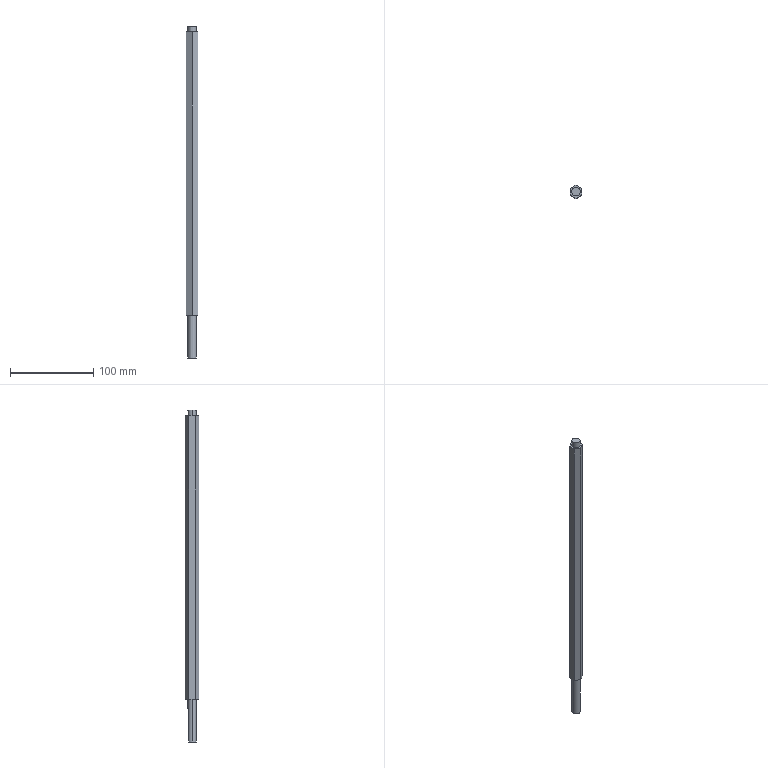Part | STEP file | 602-12-0050 | 1 solid | 16 faces | box 14 x 16.166 x 398 mm | volume 62104 mm3 | plane 12 | cylinder 4 | commonest cylinder face diameters 10 x4
STEP:
#1=CARTESIAN_POINT('',(0.,0.,0.));
#2=DIRECTION('',(0.,0.,1.));
#3=DIRECTION('',(1.,0.,0.));
#4=AXIS2_PLACEMENT_3D('',#1,#2,#3);
#5=CARTESIAN_POINT('',(-5.,0.,-51.));
#6=VERTEX_POINT('',#5);
#7=CARTESIAN_POINT('',(-3.,4.,-51.));
#8=VERTEX_POINT('',#7);
#9=CARTESIAN_POINT('',(0.,0.,-51.));
#10=DIRECTION('',(0.,0.,-1.));
#11=DIRECTION('',(-1.,0.,0.));
#12=AXIS2_PLACEMENT_3D('',#9,#10,#11);
#13=CIRCLE('',#12,5.);
#14=CARTESIAN_POINT('',(0.,0.,-51.));
#15=DIRECTION('',(0.,0.,1.));
#16=DIRECTION('',(1.,0.,0.));
#17=AXIS2_PLACEMENT_3D('',#14,#15,#16);
#18=CYLINDRICAL_SURFACE('',#17,5.);
#19=CARTESIAN_POINT('',(3.142,0.));
#20=DIRECTION('',(-1.,0.));
#21=VECTOR('',#20,1.);
#22=LINE('',#19,#21);
#23=(GEOMETRIC_REPRESENTATION_CONTEXT(2)PARAMETRIC_REPRESENTATION_CONTEXT()REPRESENTATION_CONTEXT('',''));
#24=DEFINITIONAL_REPRESENTATION('',(#22),#23);
#25=PCURVE('',#18,#24);
#26=CARTESIAN_POINT('',(0.,0.,-51.));
#27=DIRECTION('',(0.,0.,-1.));
#28=DIRECTION('',(-1.,0.,0.));
#29=AXIS2_PLACEMENT_3D('',#26,#27,#28);
#30=PLANE('',#29);
#31=CARTESIAN_POINT('',(0.,0.));
#32=DIRECTION('',(1.,0.));
#33=AXIS2_PLACEMENT_2D('',#31,#32);
#34=CIRCLE('',#33,5.);
#35=(GEOMETRIC_REPRESENTATION_CONTEXT(2)PARAMETRIC_REPRESENTATION_CONTEXT()REPRESENTATION_CONTEXT('',''));
#36=DEFINITIONAL_REPRESENTATION('',(#34),#35);
#37=PCURVE('',#30,#36);
#38=SURFACE_CURVE('',#13,(#25,#37),.PCURVE_S1.);
#39=EDGE_CURVE('',#6,#8,#38,.T.);
#40=ORIENTED_EDGE('',*,*,#39,.F.);
#41=CARTESIAN_POINT('',(-5.,0.,0.));
#42=VERTEX_POINT('',#41);
#43=CARTESIAN_POINT('',(-5.,0.,-51.));
#44=DIRECTION('',(0.,0.,1.));
#45=VECTOR('',#44,1.);
#46=LINE('',#43,#45);
#47=CARTESIAN_POINT('',(3.142,0.));
#48=DIRECTION('',(0.,1.));
#49=VECTOR('',#48,1.);
#50=LINE('',#47,#49);
#51=(GEOMETRIC_REPRESENTATION_CONTEXT(2)PARAMETRIC_REPRESENTATION_CONTEXT()REPRESENTATION_CONTEXT('',''));
#52=DEFINITIONAL_REPRESENTATION('',(#50),#51);
#53=PCURVE('',#18,#52);
#54=CARTESIAN_POINT('',(0.,0.,-51.));
#55=DIRECTION('',(0.,0.,1.));
#56=DIRECTION('',(1.,0.,0.));
#57=AXIS2_PLACEMENT_3D('',#54,#55,#56);
#58=CYLINDRICAL_SURFACE('',#57,5.);
#59=CARTESIAN_POINT('',(3.142,0.));
#60=DIRECTION('',(0.,1.));
#61=VECTOR('',#60,1.);
#62=LINE('',#59,#61);
#63=(GEOMETRIC_REPRESENTATION_CONTEXT(2)PARAMETRIC_REPRESENTATION_CONTEXT()REPRESENTATION_CONTEXT('',''));
#64=DEFINITIONAL_REPRESENTATION('',(#62),#63);
#65=PCURVE('',#58,#64);
#66=SURFACE_CURVE('',#46,(#53,#65),.PCURVE_S1.);
#67=EDGE_CURVE('',#6,#42,#66,.T.);
#68=ORIENTED_EDGE('',*,*,#67,.T.);
#69=CARTESIAN_POINT('',(5.,0.,0.));
#70=VERTEX_POINT('',#69);
#71=CARTESIAN_POINT('',(0.,0.,0.));
#72=DIRECTION('',(0.,0.,-1.));
#73=DIRECTION('',(1.,0.,0.));
#74=AXIS2_PLACEMENT_3D('',#71,#72,#73);
#75=CIRCLE('',#74,5.);
#76=CARTESIAN_POINT('',(6.283,51.));
#77=DIRECTION('',(-1.,0.));
#78=VECTOR('',#77,1.);
#79=LINE('',#76,#78);
#80=(GEOMETRIC_REPRESENTATION_CONTEXT(2)PARAMETRIC_REPRESENTATION_CONTEXT()REPRESENTATION_CONTEXT('',''));
#81=DEFINITIONAL_REPRESENTATION('',(#79),#80);
#82=PCURVE('',#18,#81);
#83=CARTESIAN_POINT('',(0.,0.,0.));
#84=DIRECTION('',(0.,0.,1.));
#85=DIRECTION('',(1.,0.,0.));
#86=AXIS2_PLACEMENT_3D('',#83,#84,#85);
#87=PLANE('',#86);
#88=CARTESIAN_POINT('',(5.,0.));
#89=CARTESIAN_POINT('',(5.,-8.66));
#90=CARTESIAN_POINT('',(-2.5,-4.33));
#91=CARTESIAN_POINT('',(-10.,0.));
#92=CARTESIAN_POINT('',(-2.5,4.33));
#93=CARTESIAN_POINT('',(5.,8.66));
#94=CARTESIAN_POINT('',(5.,0.));
#95=(BOUNDED_CURVE()B_SPLINE_CURVE(2,(#88,#89,#90,#91,#92,#93,#94),.UNSPECIFIED.,.T.,.F.)B_SPLINE_CURVE_WITH_KNOTS((1,2,2,2,2,1),(-2.094,0.,2.094,4.189,6.283,8.378),.UNSPECIFIED.)CURVE()GEOMETRIC_REPRESENTATION_ITEM()RATIONAL_B_SPLINE_CURVE((1.,0.5,1.,0.5,1.,0.5,1.))REPRESENTATION_ITEM(''));
#96=(GEOMETRIC_REPRESENTATION_CONTEXT(2)PARAMETRIC_REPRESENTATION_CONTEXT()REPRESENTATION_CONTEXT('',''));
#97=DEFINITIONAL_REPRESENTATION('',(#95),#96);
#98=PCURVE('',#87,#97);
#99=SURFACE_CURVE('',#75,(#82,#98),.PCURVE_S1.);
#100=EDGE_CURVE('',#42,#70,#99,.T.);
#101=ORIENTED_EDGE('',*,*,#100,.T.);
#102=CARTESIAN_POINT('',(5.,0.,-51.));
#103=VERTEX_POINT('',#102);
#104=CARTESIAN_POINT('',(5.,0.,-51.));
#105=DIRECTION('',(0.,0.,1.));
#106=VECTOR('',#105,1.);
#107=LINE('',#104,#106);
#108=CARTESIAN_POINT('',(0.,0.));
#109=DIRECTION('',(0.,1.));
#110=VECTOR('',#109,1.);
#111=LINE('',#108,#110);
#112=(GEOMETRIC_REPRESENTATION_CONTEXT(2)PARAMETRIC_REPRESENTATION_CONTEXT()REPRESENTATION_CONTEXT('',''));
#113=DEFINITIONAL_REPRESENTATION('',(#111),#112);
#114=PCURVE('',#18,#113);
#115=CARTESIAN_POINT('',(6.283,0.));
#116=DIRECTION('',(0.,1.));
#117=VECTOR('',#116,1.);
#118=LINE('',#115,#117);
#119=(GEOMETRIC_REPRESENTATION_CONTEXT(2)PARAMETRIC_REPRESENTATION_CONTEXT()REPRESENTATION_CONTEXT('',''));
#120=DEFINITIONAL_REPRESENTATION('',(#118),#119);
#121=PCURVE('',#58,#120);
#122=SURFACE_CURVE('',#107,(#114,#121),.PCURVE_S1.);
#123=EDGE_CURVE('',#103,#70,#122,.T.);
#124=ORIENTED_EDGE('',*,*,#123,.F.);
#125=CARTESIAN_POINT('',(3.,4.,-51.));
#126=VERTEX_POINT('',#125);
#127=CARTESIAN_POINT('',(0.,0.,-51.));
#128=DIRECTION('',(0.,0.,-1.));
#129=DIRECTION('',(-1.,0.,0.));
#130=AXIS2_PLACEMENT_3D('',#127,#128,#129);
#131=CIRCLE('',#130,5.);
#132=CARTESIAN_POINT('',(3.142,0.));
#133=DIRECTION('',(-1.,0.));
#134=VECTOR('',#133,1.);
#135=LINE('',#132,#134);
#136=(GEOMETRIC_REPRESENTATION_CONTEXT(2)PARAMETRIC_REPRESENTATION_CONTEXT()REPRESENTATION_CONTEXT('',''));
#137=DEFINITIONAL_REPRESENTATION('',(#135),#136);
#138=PCURVE('',#18,#137);
#139=CARTESIAN_POINT('',(0.,0.));
#140=DIRECTION('',(1.,0.));
#141=AXIS2_PLACEMENT_2D('',#139,#140);
#142=CIRCLE('',#141,5.);
#143=(GEOMETRIC_REPRESENTATION_CONTEXT(2)PARAMETRIC_REPRESENTATION_CONTEXT()REPRESENTATION_CONTEXT('',''));
#144=DEFINITIONAL_REPRESENTATION('',(#142),#143);
#145=PCURVE('',#30,#144);
#146=SURFACE_CURVE('',#131,(#138,#145),.PCURVE_S1.);
#147=EDGE_CURVE('',#126,#103,#146,.T.);
#148=ORIENTED_EDGE('',*,*,#147,.F.);
#149=CARTESIAN_POINT('',(3.,4.,-11.));
#150=VERTEX_POINT('',#149);
#151=CARTESIAN_POINT('',(3.,4.,-11.));
#152=DIRECTION('',(0.,0.,-1.));
#153=VECTOR('',#152,1.);
#154=LINE('',#151,#153);
#155=CARTESIAN_POINT('',(0.9273,40.));
#156=DIRECTION('',(0.,-1.));
#157=VECTOR('',#156,1.);
#158=LINE('',#155,#157);
#159=(GEOMETRIC_REPRESENTATION_CONTEXT(2)PARAMETRIC_REPRESENTATION_CONTEXT()REPRESENTATION_CONTEXT('',''));
#160=DEFINITIONAL_REPRESENTATION('',(#158),#159);
#161=PCURVE('',#18,#160);
#162=CARTESIAN_POINT('',(3.,4.,-11.));
#163=DIRECTION('',(0.,-1.,0.));
#164=DIRECTION('',(0.,0.,-1.));
#165=AXIS2_PLACEMENT_3D('',#162,#163,#164);
#166=PLANE('',#165);
#167=CARTESIAN_POINT('',(0.,0.));
#168=DIRECTION('',(1.,0.));
#169=VECTOR('',#168,1.);
#170=LINE('',#167,#169);
#171=(GEOMETRIC_REPRESENTATION_CONTEXT(2)PARAMETRIC_REPRESENTATION_CONTEXT()REPRESENTATION_CONTEXT('',''));
#172=DEFINITIONAL_REPRESENTATION('',(#170),#171);
#173=PCURVE('',#166,#172);
#174=SURFACE_CURVE('',#154,(#161,#173),.PCURVE_S1.);
#175=EDGE_CURVE('',#150,#126,#174,.T.);
#176=ORIENTED_EDGE('',*,*,#175,.F.);
#177=CARTESIAN_POINT('',(-3.,4.,-11.));
#178=VERTEX_POINT('',#177);
#179=CARTESIAN_POINT('',(0.,0.,-11.));
#180=DIRECTION('',(0.,0.,-1.));
#181=DIRECTION('',(-1.,0.,0.));
#182=AXIS2_PLACEMENT_3D('',#179,#180,#181);
#183=CIRCLE('',#182,5.);
#184=CARTESIAN_POINT('',(3.142,40.));
#185=DIRECTION('',(-1.,0.));
#186=VECTOR('',#185,1.);
#187=LINE('',#184,#186);
#188=(GEOMETRIC_REPRESENTATION_CONTEXT(2)PARAMETRIC_REPRESENTATION_CONTEXT()REPRESENTATION_CONTEXT('',''));
#189=DEFINITIONAL_REPRESENTATION('',(#187),#188);
#190=PCURVE('',#18,#189);
#191=CARTESIAN_POINT('',(0.,0.,-11.));
#192=DIRECTION('',(0.,0.,-1.));
#193=DIRECTION('',(-1.,0.,0.));
#194=AXIS2_PLACEMENT_3D('',#191,#192,#193);
#195=PLANE('',#194);
#196=CARTESIAN_POINT('',(0.,0.));
#197=DIRECTION('',(1.,0.));
#198=AXIS2_PLACEMENT_2D('',#196,#197);
#199=CIRCLE('',#198,5.);
#200=(GEOMETRIC_REPRESENTATION_CONTEXT(2)PARAMETRIC_REPRESENTATION_CONTEXT()REPRESENTATION_CONTEXT('',''));
#201=DEFINITIONAL_REPRESENTATION('',(#199),#200);
#202=PCURVE('',#195,#201);
#203=SURFACE_CURVE('',#183,(#190,#202),.PCURVE_S1.);
#204=EDGE_CURVE('',#178,#150,#203,.T.);
#205=ORIENTED_EDGE('',*,*,#204,.F.);
#206=CARTESIAN_POINT('',(-3.,4.,-11.));
#207=DIRECTION('',(0.,0.,-1.));
#208=VECTOR('',#207,1.);
#209=LINE('',#206,#208);
#210=CARTESIAN_POINT('',(2.214,40.));
#211=DIRECTION('',(0.,-1.));
#212=VECTOR('',#211,1.);
#213=LINE('',#210,#212);
#214=(GEOMETRIC_REPRESENTATION_CONTEXT(2)PARAMETRIC_REPRESENTATION_CONTEXT()REPRESENTATION_CONTEXT('',''));
#215=DEFINITIONAL_REPRESENTATION('',(#213),#214);
#216=PCURVE('',#18,#215);
#217=CARTESIAN_POINT('',(0.,-6.));
#218=DIRECTION('',(1.,0.));
#219=VECTOR('',#218,1.);
#220=LINE('',#217,#219);
#221=(GEOMETRIC_REPRESENTATION_CONTEXT(2)PARAMETRIC_REPRESENTATION_CONTEXT()REPRESENTATION_CONTEXT('',''));
#222=DEFINITIONAL_REPRESENTATION('',(#220),#221);
#223=PCURVE('',#166,#222);
#224=SURFACE_CURVE('',#209,(#216,#223),.PCURVE_S1.);
#225=EDGE_CURVE('',#178,#8,#224,.T.);
#226=ORIENTED_EDGE('',*,*,#225,.T.);
#227=EDGE_LOOP('',(#40,#68,#101,#124,#148,#176,#205,#226));
#228=FACE_BOUND('',#227,.T.);
#229=ADVANCED_FACE('',(#228),#18,.T.);
#230=CARTESIAN_POINT('',(5.,0.,347.));
#231=VERTEX_POINT('',#230);
#232=CARTESIAN_POINT('',(-5.,0.,347.));
#233=VERTEX_POINT('',#232);
#234=CARTESIAN_POINT('',(0.,0.,347.));
#235=DIRECTION('',(0.,0.,1.));
#236=DIRECTION('',(1.,0.,0.));
#237=AXIS2_PLACEMENT_3D('',#234,#235,#236);
#238=CIRCLE('',#237,5.);
#239=CARTESIAN_POINT('',(0.,0.,347.));
#240=DIRECTION('',(0.,0.,-1.));
#241=DIRECTION('',(-1.,0.,0.));
#242=AXIS2_PLACEMENT_3D('',#239,#240,#241);
#243=CYLINDRICAL_SURFACE('',#242,5.);
#244=CARTESIAN_POINT('',(3.142,0.));
#245=DIRECTION('',(-1.,0.));
#246=VECTOR('',#245,1.);
#247=LINE('',#244,#246);
#248=(GEOMETRIC_REPRESENTATION_CONTEXT(2)PARAMETRIC_REPRESENTATION_CONTEXT()REPRESENTATION_CONTEXT('',''));
#249=DEFINITIONAL_REPRESENTATION('',(#247),#248);
#250=PCURVE('',#243,#249);
#251=CARTESIAN_POINT('',(0.,0.,347.));
#252=DIRECTION('',(0.,0.,1.));
#253=DIRECTION('',(1.,0.,0.));
#254=AXIS2_PLACEMENT_3D('',#251,#252,#253);
#255=PLANE('',#254);
#256=CARTESIAN_POINT('',(0.,0.));
#257=DIRECTION('',(1.,0.));
#258=AXIS2_PLACEMENT_2D('',#256,#257);
#259=CIRCLE('',#258,5.);
#260=(GEOMETRIC_REPRESENTATION_CONTEXT(2)PARAMETRIC_REPRESENTATION_CONTEXT()REPRESENTATION_CONTEXT('',''));
#261=DEFINITIONAL_REPRESENTATION('',(#259),#260);
#262=PCURVE('',#255,#261);
#263=SURFACE_CURVE('',#238,(#250,#262),.PCURVE_S1.);
#264=EDGE_CURVE('',#231,#233,#263,.T.);
#265=ORIENTED_EDGE('',*,*,#264,.F.);
#266=CARTESIAN_POINT('',(5.,0.,340.));
#267=VERTEX_POINT('',#266);
#268=CARTESIAN_POINT('',(5.,0.,347.));
#269=DIRECTION('',(0.,0.,-1.));
#270=VECTOR('',#269,1.);
#271=LINE('',#268,#270);
#272=CARTESIAN_POINT('',(3.142,0.));
#273=DIRECTION('',(0.,1.));
#274=VECTOR('',#273,1.);
#275=LINE('',#272,#274);
#276=(GEOMETRIC_REPRESENTATION_CONTEXT(2)PARAMETRIC_REPRESENTATION_CONTEXT()REPRESENTATION_CONTEXT('',''));
#277=DEFINITIONAL_REPRESENTATION('',(#275),#276);
#278=PCURVE('',#243,#277);
#279=CARTESIAN_POINT('',(0.,0.,347.));
#280=DIRECTION('',(0.,0.,-1.));
#281=DIRECTION('',(-1.,0.,0.));
#282=AXIS2_PLACEMENT_3D('',#279,#280,#281);
#283=CYLINDRICAL_SURFACE('',#282,5.);
#284=CARTESIAN_POINT('',(3.142,0.));
#285=DIRECTION('',(0.,1.));
#286=VECTOR('',#285,1.);
#287=LINE('',#284,#286);
#288=(GEOMETRIC_REPRESENTATION_CONTEXT(2)PARAMETRIC_REPRESENTATION_CONTEXT()REPRESENTATION_CONTEXT('',''));
#289=DEFINITIONAL_REPRESENTATION('',(#287),#288);
#290=PCURVE('',#283,#289);
#291=SURFACE_CURVE('',#271,(#278,#290),.PCURVE_S1.);
#292=EDGE_CURVE('',#231,#267,#291,.T.);
#293=ORIENTED_EDGE('',*,*,#292,.T.);
#294=CARTESIAN_POINT('',(-5.,0.,340.));
#295=VERTEX_POINT('',#294);
#296=CARTESIAN_POINT('',(0.,0.,340.));
#297=DIRECTION('',(0.,0.,1.));
#298=DIRECTION('',(1.,0.,0.));
#299=AXIS2_PLACEMENT_3D('',#296,#297,#298);
#300=CIRCLE('',#299,5.);
#301=CARTESIAN_POINT('',(3.142,7.));
#302=DIRECTION('',(-1.,0.));
#303=VECTOR('',#302,1.);
#304=LINE('',#301,#303);
#305=(GEOMETRIC_REPRESENTATION_CONTEXT(2)PARAMETRIC_REPRESENTATION_CONTEXT()REPRESENTATION_CONTEXT('',''));
#306=DEFINITIONAL_REPRESENTATION('',(#304),#305);
#307=PCURVE('',#243,#306);
#308=CARTESIAN_POINT('',(0.,0.,340.));
#309=DIRECTION('',(0.,0.,1.));
#310=DIRECTION('',(1.,0.,0.));
#311=AXIS2_PLACEMENT_3D('',#308,#309,#310);
#312=PLANE('',#311);
#313=CARTESIAN_POINT('',(0.,0.));
#314=DIRECTION('',(1.,0.));
#315=AXIS2_PLACEMENT_2D('',#313,#314);
#316=CIRCLE('',#315,5.);
#317=(GEOMETRIC_REPRESENTATION_CONTEXT(2)PARAMETRIC_REPRESENTATION_CONTEXT()REPRESENTATION_CONTEXT('',''));
#318=DEFINITIONAL_REPRESENTATION('',(#316),#317);
#319=PCURVE('',#312,#318);
#320=SURFACE_CURVE('',#300,(#307,#319),.PCURVE_S1.);
#321=EDGE_CURVE('',#267,#295,#320,.T.);
#322=ORIENTED_EDGE('',*,*,#321,.T.);
#323=CARTESIAN_POINT('',(-5.,0.,347.));
#324=DIRECTION('',(0.,0.,-1.));
#325=VECTOR('',#324,1.);
#326=LINE('',#323,#325);
#327=CARTESIAN_POINT('',(0.,0.));
#328=DIRECTION('',(0.,1.));
#329=VECTOR('',#328,1.);
#330=LINE('',#327,#329);
#331=(GEOMETRIC_REPRESENTATION_CONTEXT(2)PARAMETRIC_REPRESENTATION_CONTEXT()REPRESENTATION_CONTEXT('',''));
#332=DEFINITIONAL_REPRESENTATION('',(#330),#331);
#333=PCURVE('',#243,#332);
#334=CARTESIAN_POINT('',(6.283,0.));
#335=DIRECTION('',(0.,1.));
#336=VECTOR('',#335,1.);
#337=LINE('',#334,#336);
#338=(GEOMETRIC_REPRESENTATION_CONTEXT(2)PARAMETRIC_REPRESENTATION_CONTEXT()REPRESENTATION_CONTEXT('',''));
#339=DEFINITIONAL_REPRESENTATION('',(#337),#338);
#340=PCURVE('',#283,#339);
#341=SURFACE_CURVE('',#326,(#333,#340),.PCURVE_S1.);
#342=EDGE_CURVE('',#233,#295,#341,.T.);
#343=ORIENTED_EDGE('',*,*,#342,.F.);
#344=EDGE_LOOP('',(#265,#293,#322,#343));
#345=FACE_BOUND('',#344,.T.);
#346=ADVANCED_FACE('',(#345),#243,.T.);
#347=CARTESIAN_POINT('',(7.,4.041,0.));
#348=VERTEX_POINT('',#347);
#349=CARTESIAN_POINT('',(0.,8.083,0.));
#350=VERTEX_POINT('',#349);
#351=CARTESIAN_POINT('',(7.,4.041,0.));
#352=DIRECTION('',(-0.866,0.5,0.));
#353=VECTOR('',#352,1.);
#354=LINE('',#351,#353);
#355=CARTESIAN_POINT('',(7.,4.041));
#356=DIRECTION('',(-0.866,0.5));
#357=VECTOR('',#356,1.);
#358=LINE('',#355,#357);
#359=(GEOMETRIC_REPRESENTATION_CONTEXT(2)PARAMETRIC_REPRESENTATION_CONTEXT()REPRESENTATION_CONTEXT('',''));
#360=DEFINITIONAL_REPRESENTATION('',(#358),#359);
#361=PCURVE('',#87,#360);
#362=CARTESIAN_POINT('',(7.,4.041,340.));
#363=DIRECTION('',(-0.5,-0.866,0.));
#364=DIRECTION('',(0.866,-0.5,0.));
#365=AXIS2_PLACEMENT_3D('',#362,#363,#364);
#366=PLANE('',#365);
#367=CARTESIAN_POINT('',(0.,-340.));
#368=DIRECTION('',(-1.,0.));
#369=VECTOR('',#368,1.);
#370=LINE('',#367,#369);
#371=(GEOMETRIC_REPRESENTATION_CONTEXT(2)PARAMETRIC_REPRESENTATION_CONTEXT()REPRESENTATION_CONTEXT('',''));
#372=DEFINITIONAL_REPRESENTATION('',(#370),#371);
#373=PCURVE('',#366,#372);
#374=SURFACE_CURVE('',#354,(#361,#373),.PCURVE_S1.);
#375=EDGE_CURVE('',#348,#350,#374,.T.);
#376=ORIENTED_EDGE('',*,*,#375,.F.);
#377=CARTESIAN_POINT('',(7.,-4.041,0.));
#378=VERTEX_POINT('',#377);
#379=CARTESIAN_POINT('',(7.,-4.041,0.));
#380=DIRECTION('',(0.,1.,0.));
#381=VECTOR('',#380,1.);
#382=LINE('',#379,#381);
#383=CARTESIAN_POINT('',(7.,-4.041));
#384=DIRECTION('',(0.,1.));
#385=VECTOR('',#384,1.);
#386=LINE('',#383,#385);
#387=(GEOMETRIC_REPRESENTATION_CONTEXT(2)PARAMETRIC_REPRESENTATION_CONTEXT()REPRESENTATION_CONTEXT('',''));
#388=DEFINITIONAL_REPRESENTATION('',(#386),#387);
#389=PCURVE('',#87,#388);
#390=CARTESIAN_POINT('',(7.,-4.041,340.));
#391=DIRECTION('',(-1.,0.,0.));
#392=DIRECTION('',(0.,0.,1.));
#393=AXIS2_PLACEMENT_3D('',#390,#391,#392);
#394=PLANE('',#393);
#395=CARTESIAN_POINT('',(-340.,0.));
#396=DIRECTION('',(0.,1.));
#397=VECTOR('',#396,1.);
#398=LINE('',#395,#397);
#399=(GEOMETRIC_REPRESENTATION_CONTEXT(2)PARAMETRIC_REPRESENTATION_CONTEXT()REPRESENTATION_CONTEXT('',''));
#400=DEFINITIONAL_REPRESENTATION('',(#398),#399);
#401=PCURVE('',#394,#400);
#402=SURFACE_CURVE('',#382,(#389,#401),.PCURVE_S1.);
#403=EDGE_CURVE('',#378,#348,#402,.T.);
#404=ORIENTED_EDGE('',*,*,#403,.F.);
#405=CARTESIAN_POINT('',(0.,-8.083,0.));
#406=VERTEX_POINT('',#405);
#407=CARTESIAN_POINT('',(0.,-8.083,0.));
#408=DIRECTION('',(0.866,0.5,0.));
#409=VECTOR('',#408,1.);
#410=LINE('',#407,#409);
#411=CARTESIAN_POINT('',(0.,-8.083));
#412=DIRECTION('',(0.866,0.5));
#413=VECTOR('',#412,1.);
#414=LINE('',#411,#413);
#415=(GEOMETRIC_REPRESENTATION_CONTEXT(2)PARAMETRIC_REPRESENTATION_CONTEXT()REPRESENTATION_CONTEXT('',''));
#416=DEFINITIONAL_REPRESENTATION('',(#414),#415);
#417=PCURVE('',#87,#416);
#418=CARTESIAN_POINT('',(0.,-8.083,340.));
#419=DIRECTION('',(-0.5,0.866,0.));
#420=DIRECTION('',(-0.866,-0.5,0.));
#421=AXIS2_PLACEMENT_3D('',#418,#419,#420);
#422=PLANE('',#421);
#423=CARTESIAN_POINT('',(0.,-340.));
#424=DIRECTION('',(-1.,0.));
#425=VECTOR('',#424,1.);
#426=LINE('',#423,#425);
#427=(GEOMETRIC_REPRESENTATION_CONTEXT(2)PARAMETRIC_REPRESENTATION_CONTEXT()REPRESENTATION_CONTEXT('',''));
#428=DEFINITIONAL_REPRESENTATION('',(#426),#427);
#429=PCURVE('',#422,#428);
#430=SURFACE_CURVE('',#410,(#417,#429),.PCURVE_S1.);
#431=EDGE_CURVE('',#406,#378,#430,.T.);
#432=ORIENTED_EDGE('',*,*,#431,.F.);
#433=CARTESIAN_POINT('',(-7.,-4.041,0.));
#434=VERTEX_POINT('',#433);
#435=CARTESIAN_POINT('',(-7.,-4.041,0.));
#436=DIRECTION('',(0.866,-0.5,0.));
#437=VECTOR('',#436,1.);
#438=LINE('',#435,#437);
#439=CARTESIAN_POINT('',(-7.,-4.041));
#440=DIRECTION('',(0.866,-0.5));
#441=VECTOR('',#440,1.);
#442=LINE('',#439,#441);
#443=(GEOMETRIC_REPRESENTATION_CONTEXT(2)PARAMETRIC_REPRESENTATION_CONTEXT()REPRESENTATION_CONTEXT('',''));
#444=DEFINITIONAL_REPRESENTATION('',(#442),#443);
#445=PCURVE('',#87,#444);
#446=CARTESIAN_POINT('',(-7.,-4.041,340.));
#447=DIRECTION('',(0.5,0.866,0.));
#448=DIRECTION('',(-0.866,0.5,0.));
#449=AXIS2_PLACEMENT_3D('',#446,#447,#448);
#450=PLANE('',#449);
#451=CARTESIAN_POINT('',(0.,-340.));
#452=DIRECTION('',(-1.,0.));
#453=VECTOR('',#452,1.);
#454=LINE('',#451,#453);
#455=(GEOMETRIC_REPRESENTATION_CONTEXT(2)PARAMETRIC_REPRESENTATION_CONTEXT()REPRESENTATION_CONTEXT('',''));
#456=DEFINITIONAL_REPRESENTATION('',(#454),#455);
#457=PCURVE('',#450,#456);
#458=SURFACE_CURVE('',#438,(#445,#457),.PCURVE_S1.);
#459=EDGE_CURVE('',#434,#406,#458,.T.);
#460=ORIENTED_EDGE('',*,*,#459,.F.);
#461=CARTESIAN_POINT('',(-7.,4.041,0.));
#462=VERTEX_POINT('',#461);
#463=CARTESIAN_POINT('',(-7.,4.041,0.));
#464=DIRECTION('',(0.,-1.,0.));
#465=VECTOR('',#464,1.);
#466=LINE('',#463,#465);
#467=CARTESIAN_POINT('',(-7.,4.041));
#468=DIRECTION('',(0.,-1.));
#469=VECTOR('',#468,1.);
#470=LINE('',#467,#469);
#471=(GEOMETRIC_REPRESENTATION_CONTEXT(2)PARAMETRIC_REPRESENTATION_CONTEXT()REPRESENTATION_CONTEXT('',''));
#472=DEFINITIONAL_REPRESENTATION('',(#470),#471);
#473=PCURVE('',#87,#472);
#474=CARTESIAN_POINT('',(-7.,4.041,340.));
#475=DIRECTION('',(1.,0.,0.));
#476=DIRECTION('',(0.,0.,-1.));
#477=AXIS2_PLACEMENT_3D('',#474,#475,#476);
#478=PLANE('',#477);
#479=CARTESIAN_POINT('',(340.,0.));
#480=DIRECTION('',(0.,-1.));
#481=VECTOR('',#480,1.);
#482=LINE('',#479,#481);
#483=(GEOMETRIC_REPRESENTATION_CONTEXT(2)PARAMETRIC_REPRESENTATION_CONTEXT()REPRESENTATION_CONTEXT('',''));
#484=DEFINITIONAL_REPRESENTATION('',(#482),#483);
#485=PCURVE('',#478,#484);
#486=SURFACE_CURVE('',#466,(#473,#485),.PCURVE_S1.);
#487=EDGE_CURVE('',#462,#434,#486,.T.);
#488=ORIENTED_EDGE('',*,*,#487,.F.);
#489=CARTESIAN_POINT('',(0.,8.083,0.));
#490=DIRECTION('',(-0.866,-0.5,0.));
#491=VECTOR('',#490,1.);
#492=LINE('',#489,#491);
#493=CARTESIAN_POINT('',(0.,8.083));
#494=DIRECTION('',(-0.866,-0.5));
#495=VECTOR('',#494,1.);
#496=LINE('',#493,#495);
#497=(GEOMETRIC_REPRESENTATION_CONTEXT(2)PARAMETRIC_REPRESENTATION_CONTEXT()REPRESENTATION_CONTEXT('',''));
#498=DEFINITIONAL_REPRESENTATION('',(#496),#497);
#499=PCURVE('',#87,#498);
#500=CARTESIAN_POINT('',(0.,8.083,340.));
#501=DIRECTION('',(0.5,-0.866,0.));
#502=DIRECTION('',(0.866,0.5,0.));
#503=AXIS2_PLACEMENT_3D('',#500,#501,#502);
#504=PLANE('',#503);
#505=CARTESIAN_POINT('',(0.,-340.));
#506=DIRECTION('',(-1.,0.));
#507=VECTOR('',#506,1.);
#508=LINE('',#505,#507);
#509=(GEOMETRIC_REPRESENTATION_CONTEXT(2)PARAMETRIC_REPRESENTATION_CONTEXT()REPRESENTATION_CONTEXT('',''));
#510=DEFINITIONAL_REPRESENTATION('',(#508),#509);
#511=PCURVE('',#504,#510);
#512=SURFACE_CURVE('',#492,(#499,#511),.PCURVE_S1.);
#513=EDGE_CURVE('',#350,#462,#512,.T.);
#514=ORIENTED_EDGE('',*,*,#513,.F.);
#515=EDGE_LOOP('',(#376,#404,#432,#460,#488,#514));
#516=FACE_BOUND('',#515,.T.);
#517=CARTESIAN_POINT('',(0.,0.,0.));
#518=DIRECTION('',(0.,0.,-1.));
#519=DIRECTION('',(1.,0.,0.));
#520=AXIS2_PLACEMENT_3D('',#517,#518,#519);
#521=CIRCLE('',#520,5.);
#522=CARTESIAN_POINT('',(5.,0.));
#523=CARTESIAN_POINT('',(5.,-8.66));
#524=CARTESIAN_POINT('',(-2.5,-4.33));
#525=CARTESIAN_POINT('',(-10.,0.));
#526=CARTESIAN_POINT('',(-2.5,4.33));
#527=CARTESIAN_POINT('',(5.,8.66));
#528=CARTESIAN_POINT('',(5.,0.));
#529=(BOUNDED_CURVE()B_SPLINE_CURVE(2,(#522,#523,#524,#525,#526,#527,#528),.UNSPECIFIED.,.T.,.F.)B_SPLINE_CURVE_WITH_KNOTS((1,2,2,2,2,1),(-2.094,0.,2.094,4.189,6.283,8.378),.UNSPECIFIED.)CURVE()GEOMETRIC_REPRESENTATION_ITEM()RATIONAL_B_SPLINE_CURVE((1.,0.5,1.,0.5,1.,0.5,1.))REPRESENTATION_ITEM(''));
#530=(GEOMETRIC_REPRESENTATION_CONTEXT(2)PARAMETRIC_REPRESENTATION_CONTEXT()REPRESENTATION_CONTEXT('',''));
#531=DEFINITIONAL_REPRESENTATION('',(#529),#530);
#532=PCURVE('',#87,#531);
#533=CARTESIAN_POINT('',(6.283,51.));
#534=DIRECTION('',(-1.,0.));
#535=VECTOR('',#534,1.);
#536=LINE('',#533,#535);
#537=(GEOMETRIC_REPRESENTATION_CONTEXT(2)PARAMETRIC_REPRESENTATION_CONTEXT()REPRESENTATION_CONTEXT('',''));
#538=DEFINITIONAL_REPRESENTATION('',(#536),#537);
#539=PCURVE('',#58,#538);
#540=SURFACE_CURVE('',#521,(#532,#539),.PCURVE_S1.);
#541=EDGE_CURVE('',#70,#42,#540,.T.);
#542=ORIENTED_EDGE('',*,*,#541,.F.);
#543=ORIENTED_EDGE('',*,*,#100,.F.);
#544=EDGE_LOOP('',(#542,#543));
#545=FACE_BOUND('',#544,.T.);
#546=ADVANCED_FACE('',(#516,#545),#87,.F.);
#547=CARTESIAN_POINT('',(7.,4.041,340.));
#548=VERTEX_POINT('',#547);
#549=CARTESIAN_POINT('',(0.,8.083,340.));
#550=VERTEX_POINT('',#549);
#551=CARTESIAN_POINT('',(7.,4.041,340.));
#552=DIRECTION('',(-0.866,0.5,0.));
#553=VECTOR('',#552,1.);
#554=LINE('',#551,#553);
#555=CARTESIAN_POINT('',(7.,4.041));
#556=DIRECTION('',(-0.866,0.5));
#557=VECTOR('',#556,1.);
#558=LINE('',#555,#557);
#559=(GEOMETRIC_REPRESENTATION_CONTEXT(2)PARAMETRIC_REPRESENTATION_CONTEXT()REPRESENTATION_CONTEXT('',''));
#560=DEFINITIONAL_REPRESENTATION('',(#558),#559);
#561=PCURVE('',#312,#560);
#562=CARTESIAN_POINT('',(0.,0.));
#563=DIRECTION('',(-1.,0.));
#564=VECTOR('',#563,1.);
#565=LINE('',#562,#564);
#566=(GEOMETRIC_REPRESENTATION_CONTEXT(2)PARAMETRIC_REPRESENTATION_CONTEXT()REPRESENTATION_CONTEXT('',''));
#567=DEFINITIONAL_REPRESENTATION('',(#565),#566);
#568=PCURVE('',#366,#567);
#569=SURFACE_CURVE('',#554,(#561,#568),.PCURVE_S1.);
#570=EDGE_CURVE('',#548,#550,#569,.T.);
#571=ORIENTED_EDGE('',*,*,#570,.T.);
#572=CARTESIAN_POINT('',(-7.,4.041,340.));
#573=VERTEX_POINT('',#572);
#574=CARTESIAN_POINT('',(0.,8.083,340.));
#575=DIRECTION('',(-0.866,-0.5,0.));
#576=VECTOR('',#575,1.);
#577=LINE('',#574,#576);
#578=CARTESIAN_POINT('',(0.,8.083));
#579=DIRECTION('',(-0.866,-0.5));
#580=VECTOR('',#579,1.);
#581=LINE('',#578,#580);
#582=(GEOMETRIC_REPRESENTATION_CONTEXT(2)PARAMETRIC_REPRESENTATION_CONTEXT()REPRESENTATION_CONTEXT('',''));
#583=DEFINITIONAL_REPRESENTATION('',(#581),#582);
#584=PCURVE('',#312,#583);
#585=CARTESIAN_POINT('',(0.,0.));
#586=DIRECTION('',(-1.,0.));
#587=VECTOR('',#586,1.);
#588=LINE('',#585,#587);
#589=(GEOMETRIC_REPRESENTATION_CONTEXT(2)PARAMETRIC_REPRESENTATION_CONTEXT()REPRESENTATION_CONTEXT('',''));
#590=DEFINITIONAL_REPRESENTATION('',(#588),#589);
#591=PCURVE('',#504,#590);
#592=SURFACE_CURVE('',#577,(#584,#591),.PCURVE_S1.);
#593=EDGE_CURVE('',#550,#573,#592,.T.);
#594=ORIENTED_EDGE('',*,*,#593,.T.);
#595=CARTESIAN_POINT('',(-7.,-4.041,340.));
#596=VERTEX_POINT('',#595);
#597=CARTESIAN_POINT('',(-7.,4.041,340.));
#598=DIRECTION('',(0.,-1.,0.));
#599=VECTOR('',#598,1.);
#600=LINE('',#597,#599);
#601=CARTESIAN_POINT('',(-7.,4.041));
#602=DIRECTION('',(0.,-1.));
#603=VECTOR('',#602,1.);
#604=LINE('',#601,#603);
#605=(GEOMETRIC_REPRESENTATION_CONTEXT(2)PARAMETRIC_REPRESENTATION_CONTEXT()REPRESENTATION_CONTEXT('',''));
#606=DEFINITIONAL_REPRESENTATION('',(#604),#605);
#607=PCURVE('',#312,#606);
#608=CARTESIAN_POINT('',(0.,0.));
#609=DIRECTION('',(0.,-1.));
#610=VECTOR('',#609,1.);
#611=LINE('',#608,#610);
#612=(GEOMETRIC_REPRESENTATION_CONTEXT(2)PARAMETRIC_REPRESENTATION_CONTEXT()REPRESENTATION_CONTEXT('',''));
#613=DEFINITIONAL_REPRESENTATION('',(#611),#612);
#614=PCURVE('',#478,#613);
#615=SURFACE_CURVE('',#600,(#607,#614),.PCURVE_S1.);
#616=EDGE_CURVE('',#573,#596,#615,.T.);
#617=ORIENTED_EDGE('',*,*,#616,.T.);
#618=CARTESIAN_POINT('',(0.,-8.083,340.));
#619=VERTEX_POINT('',#618);
#620=CARTESIAN_POINT('',(-7.,-4.041,340.));
#621=DIRECTION('',(0.866,-0.5,0.));
#622=VECTOR('',#621,1.);
#623=LINE('',#620,#622);
#624=CARTESIAN_POINT('',(-7.,-4.041));
#625=DIRECTION('',(0.866,-0.5));
#626=VECTOR('',#625,1.);
#627=LINE('',#624,#626);
#628=(GEOMETRIC_REPRESENTATION_CONTEXT(2)PARAMETRIC_REPRESENTATION_CONTEXT()REPRESENTATION_CONTEXT('',''));
#629=DEFINITIONAL_REPRESENTATION('',(#627),#628);
#630=PCURVE('',#312,#629);
#631=CARTESIAN_POINT('',(0.,0.));
#632=DIRECTION('',(-1.,0.));
#633=VECTOR('',#632,1.);
#634=LINE('',#631,#633);
#635=(GEOMETRIC_REPRESENTATION_CONTEXT(2)PARAMETRIC_REPRESENTATION_CONTEXT()REPRESENTATION_CONTEXT('',''));
#636=DEFINITIONAL_REPRESENTATION('',(#634),#635);
#637=PCURVE('',#450,#636);
#638=SURFACE_CURVE('',#623,(#630,#637),.PCURVE_S1.);
#639=EDGE_CURVE('',#596,#619,#638,.T.);
#640=ORIENTED_EDGE('',*,*,#639,.T.);
#641=CARTESIAN_POINT('',(7.,-4.041,340.));
#642=VERTEX_POINT('',#641);
#643=CARTESIAN_POINT('',(0.,-8.083,340.));
#644=DIRECTION('',(0.866,0.5,0.));
#645=VECTOR('',#644,1.);
#646=LINE('',#643,#645);
#647=CARTESIAN_POINT('',(0.,-8.083));
#648=DIRECTION('',(0.866,0.5));
#649=VECTOR('',#648,1.);
#650=LINE('',#647,#649);
#651=(GEOMETRIC_REPRESENTATION_CONTEXT(2)PARAMETRIC_REPRESENTATION_CONTEXT()REPRESENTATION_CONTEXT('',''));
#652=DEFINITIONAL_REPRESENTATION('',(#650),#651);
#653=PCURVE('',#312,#652);
#654=CARTESIAN_POINT('',(0.,0.));
#655=DIRECTION('',(-1.,0.));
#656=VECTOR('',#655,1.);
#657=LINE('',#654,#656);
#658=(GEOMETRIC_REPRESENTATION_CONTEXT(2)PARAMETRIC_REPRESENTATION_CONTEXT()REPRESENTATION_CONTEXT('',''));
#659=DEFINITIONAL_REPRESENTATION('',(#657),#658);
#660=PCURVE('',#422,#659);
#661=SURFACE_CURVE('',#646,(#653,#660),.PCURVE_S1.);
#662=EDGE_CURVE('',#619,#642,#661,.T.);
#663=ORIENTED_EDGE('',*,*,#662,.T.);
#664=CARTESIAN_POINT('',(7.,-4.041,340.));
#665=DIRECTION('',(0.,1.,0.));
#666=VECTOR('',#665,1.);
#667=LINE('',#664,#666);
#668=CARTESIAN_POINT('',(7.,-4.041));
#669=DIRECTION('',(0.,1.));
#670=VECTOR('',#669,1.);
#671=LINE('',#668,#670);
#672=(GEOMETRIC_REPRESENTATION_CONTEXT(2)PARAMETRIC_REPRESENTATION_CONTEXT()REPRESENTATION_CONTEXT('',''));
#673=DEFINITIONAL_REPRESENTATION('',(#671),#672);
#674=PCURVE('',#312,#673);
#675=CARTESIAN_POINT('',(0.,0.));
#676=DIRECTION('',(0.,1.));
#677=VECTOR('',#676,1.);
#678=LINE('',#675,#677);
#679=(GEOMETRIC_REPRESENTATION_CONTEXT(2)PARAMETRIC_REPRESENTATION_CONTEXT()REPRESENTATION_CONTEXT('',''));
#680=DEFINITIONAL_REPRESENTATION('',(#678),#679);
#681=PCURVE('',#394,#680);
#682=SURFACE_CURVE('',#667,(#674,#681),.PCURVE_S1.);
#683=EDGE_CURVE('',#642,#548,#682,.T.);
#684=ORIENTED_EDGE('',*,*,#683,.T.);
#685=EDGE_LOOP('',(#571,#594,#617,#640,#663,#684));
#686=FACE_BOUND('',#685,.T.);
#687=CARTESIAN_POINT('',(0.,0.,340.));
#688=DIRECTION('',(0.,0.,1.));
#689=DIRECTION('',(1.,0.,0.));
#690=AXIS2_PLACEMENT_3D('',#687,#688,#689);
#691=CIRCLE('',#690,5.);
#692=CARTESIAN_POINT('',(0.,0.));
#693=DIRECTION('',(1.,0.));
#694=AXIS2_PLACEMENT_2D('',#692,#693);
#695=CIRCLE('',#694,5.);
#696=(GEOMETRIC_REPRESENTATION_CONTEXT(2)PARAMETRIC_REPRESENTATION_CONTEXT()REPRESENTATION_CONTEXT('',''));
#697=DEFINITIONAL_REPRESENTATION('',(#695),#696);
#698=PCURVE('',#312,#697);
#699=CARTESIAN_POINT('',(9.425,7.));
#700=DIRECTION('',(-1.,0.));
#701=VECTOR('',#700,1.);
#702=LINE('',#699,#701);
#703=(GEOMETRIC_REPRESENTATION_CONTEXT(2)PARAMETRIC_REPRESENTATION_CONTEXT()REPRESENTATION_CONTEXT('',''));
#704=DEFINITIONAL_REPRESENTATION('',(#702),#703);
#705=PCURVE('',#283,#704);
#706=SURFACE_CURVE('',#691,(#698,#705),.PCURVE_S1.);
#707=EDGE_CURVE('',#295,#267,#706,.T.);
#708=ORIENTED_EDGE('',*,*,#707,.F.);
#709=ORIENTED_EDGE('',*,*,#321,.F.);
#710=EDGE_LOOP('',(#708,#709));
#711=FACE_BOUND('',#710,.T.);
#712=ADVANCED_FACE('',(#686,#711),#312,.T.);
#713=ORIENTED_EDGE('',*,*,#375,.T.);
#714=CARTESIAN_POINT('',(0.,8.083,340.));
#715=DIRECTION('',(0.,0.,-1.));
#716=VECTOR('',#715,1.);
#717=LINE('',#714,#716);
#718=CARTESIAN_POINT('',(-8.083,0.));
#719=DIRECTION('',(0.,-1.));
#720=VECTOR('',#719,1.);
#721=LINE('',#718,#720);
#722=(GEOMETRIC_REPRESENTATION_CONTEXT(2)PARAMETRIC_REPRESENTATION_CONTEXT()REPRESENTATION_CONTEXT('',''));
#723=DEFINITIONAL_REPRESENTATION('',(#721),#722);
#724=PCURVE('',#366,#723);
#725=CARTESIAN_POINT('',(0.,0.));
#726=DIRECTION('',(0.,-1.));
#727=VECTOR('',#726,1.);
#728=LINE('',#725,#727);
#729=(GEOMETRIC_REPRESENTATION_CONTEXT(2)PARAMETRIC_REPRESENTATION_CONTEXT()REPRESENTATION_CONTEXT('',''));
#730=DEFINITIONAL_REPRESENTATION('',(#728),#729);
#731=PCURVE('',#504,#730);
#732=SURFACE_CURVE('',#717,(#724,#731),.PCURVE_S1.);
#733=EDGE_CURVE('',#550,#350,#732,.T.);
#734=ORIENTED_EDGE('',*,*,#733,.F.);
#735=ORIENTED_EDGE('',*,*,#570,.F.);
#736=CARTESIAN_POINT('',(7.,4.041,340.));
#737=DIRECTION('',(0.,0.,-1.));
#738=VECTOR('',#737,1.);
#739=LINE('',#736,#738);
#740=CARTESIAN_POINT('',(0.,0.));
#741=DIRECTION('',(0.,-1.));
#742=VECTOR('',#741,1.);
#743=LINE('',#740,#742);
#744=(GEOMETRIC_REPRESENTATION_CONTEXT(2)PARAMETRIC_REPRESENTATION_CONTEXT()REPRESENTATION_CONTEXT('',''));
#745=DEFINITIONAL_REPRESENTATION('',(#743),#744);
#746=PCURVE('',#366,#745);
#747=CARTESIAN_POINT('',(0.,8.083));
#748=DIRECTION('',(-1.,0.));
#749=VECTOR('',#748,1.);
#750=LINE('',#747,#749);
#751=(GEOMETRIC_REPRESENTATION_CONTEXT(2)PARAMETRIC_REPRESENTATION_CONTEXT()REPRESENTATION_CONTEXT('',''));
#752=DEFINITIONAL_REPRESENTATION('',(#750),#751);
#753=PCURVE('',#394,#752);
#754=SURFACE_CURVE('',#739,(#746,#753),.PCURVE_S1.);
#755=EDGE_CURVE('',#548,#348,#754,.T.);
#756=ORIENTED_EDGE('',*,*,#755,.T.);
#757=EDGE_LOOP('',(#713,#734,#735,#756));
#758=FACE_BOUND('',#757,.T.);
#759=ADVANCED_FACE('',(#758),#366,.F.);
#760=ORIENTED_EDGE('',*,*,#513,.T.);
#761=CARTESIAN_POINT('',(-7.,4.041,340.));
#762=DIRECTION('',(0.,0.,-1.));
#763=VECTOR('',#762,1.);
#764=LINE('',#761,#763);
#765=CARTESIAN_POINT('',(-8.083,0.));
#766=DIRECTION('',(0.,-1.));
#767=VECTOR('',#766,1.);
#768=LINE('',#765,#767);
#769=(GEOMETRIC_REPRESENTATION_CONTEXT(2)PARAMETRIC_REPRESENTATION_CONTEXT()REPRESENTATION_CONTEXT('',''));
#770=DEFINITIONAL_REPRESENTATION('',(#768),#769);
#771=PCURVE('',#504,#770);
#772=CARTESIAN_POINT('',(0.,0.));
#773=DIRECTION('',(1.,0.));
#774=VECTOR('',#773,1.);
#775=LINE('',#772,#774);
#776=(GEOMETRIC_REPRESENTATION_CONTEXT(2)PARAMETRIC_REPRESENTATION_CONTEXT()REPRESENTATION_CONTEXT('',''));
#777=DEFINITIONAL_REPRESENTATION('',(#775),#776);
#778=PCURVE('',#478,#777);
#779=SURFACE_CURVE('',#764,(#771,#778),.PCURVE_S1.);
#780=EDGE_CURVE('',#573,#462,#779,.T.);
#781=ORIENTED_EDGE('',*,*,#780,.F.);
#782=ORIENTED_EDGE('',*,*,#593,.F.);
#783=ORIENTED_EDGE('',*,*,#733,.T.);
#784=EDGE_LOOP('',(#760,#781,#782,#783));
#785=FACE_BOUND('',#784,.T.);
#786=ADVANCED_FACE('',(#785),#504,.F.);
#787=ORIENTED_EDGE('',*,*,#487,.T.);
#788=CARTESIAN_POINT('',(-7.,-4.041,340.));
#789=DIRECTION('',(0.,0.,-1.));
#790=VECTOR('',#789,1.);
#791=LINE('',#788,#790);
#792=CARTESIAN_POINT('',(0.,-8.083));
#793=DIRECTION('',(1.,0.));
#794=VECTOR('',#793,1.);
#795=LINE('',#792,#794);
#796=(GEOMETRIC_REPRESENTATION_CONTEXT(2)PARAMETRIC_REPRESENTATION_CONTEXT()REPRESENTATION_CONTEXT('',''));
#797=DEFINITIONAL_REPRESENTATION('',(#795),#796);
#798=PCURVE('',#478,#797);
#799=CARTESIAN_POINT('',(0.,0.));
#800=DIRECTION('',(0.,-1.));
#801=VECTOR('',#800,1.);
#802=LINE('',#799,#801);
#803=(GEOMETRIC_REPRESENTATION_CONTEXT(2)PARAMETRIC_REPRESENTATION_CONTEXT()REPRESENTATION_CONTEXT('',''));
#804=DEFINITIONAL_REPRESENTATION('',(#802),#803);
#805=PCURVE('',#450,#804);
#806=SURFACE_CURVE('',#791,(#798,#805),.PCURVE_S1.);
#807=EDGE_CURVE('',#596,#434,#806,.T.);
#808=ORIENTED_EDGE('',*,*,#807,.F.);
#809=ORIENTED_EDGE('',*,*,#616,.F.);
#810=ORIENTED_EDGE('',*,*,#780,.T.);
#811=EDGE_LOOP('',(#787,#808,#809,#810));
#812=FACE_BOUND('',#811,.T.);
#813=ADVANCED_FACE('',(#812),#478,.F.);
#814=ORIENTED_EDGE('',*,*,#459,.T.);
#815=CARTESIAN_POINT('',(0.,-8.083,340.));
#816=DIRECTION('',(0.,0.,-1.));
#817=VECTOR('',#816,1.);
#818=LINE('',#815,#817);
#819=CARTESIAN_POINT('',(-8.083,0.));
#820=DIRECTION('',(0.,-1.));
#821=VECTOR('',#820,1.);
#822=LINE('',#819,#821);
#823=(GEOMETRIC_REPRESENTATION_CONTEXT(2)PARAMETRIC_REPRESENTATION_CONTEXT()REPRESENTATION_CONTEXT('',''));
#824=DEFINITIONAL_REPRESENTATION('',(#822),#823);
#825=PCURVE('',#450,#824);
#826=CARTESIAN_POINT('',(0.,0.));
#827=DIRECTION('',(0.,-1.));
#828=VECTOR('',#827,1.);
#829=LINE('',#826,#828);
#830=(GEOMETRIC_REPRESENTATION_CONTEXT(2)PARAMETRIC_REPRESENTATION_CONTEXT()REPRESENTATION_CONTEXT('',''));
#831=DEFINITIONAL_REPRESENTATION('',(#829),#830);
#832=PCURVE('',#422,#831);
#833=SURFACE_CURVE('',#818,(#825,#832),.PCURVE_S1.);
#834=EDGE_CURVE('',#619,#406,#833,.T.);
#835=ORIENTED_EDGE('',*,*,#834,.F.);
#836=ORIENTED_EDGE('',*,*,#639,.F.);
#837=ORIENTED_EDGE('',*,*,#807,.T.);
#838=EDGE_LOOP('',(#814,#835,#836,#837));
#839=FACE_BOUND('',#838,.T.);
#840=ADVANCED_FACE('',(#839),#450,.F.);
#841=ORIENTED_EDGE('',*,*,#431,.T.);
#842=CARTESIAN_POINT('',(7.,-4.041,340.));
#843=DIRECTION('',(0.,0.,-1.));
#844=VECTOR('',#843,1.);
#845=LINE('',#842,#844);
#846=CARTESIAN_POINT('',(-8.083,0.));
#847=DIRECTION('',(0.,-1.));
#848=VECTOR('',#847,1.);
#849=LINE('',#846,#848);
#850=(GEOMETRIC_REPRESENTATION_CONTEXT(2)PARAMETRIC_REPRESENTATION_CONTEXT()REPRESENTATION_CONTEXT('',''));
#851=DEFINITIONAL_REPRESENTATION('',(#849),#850);
#852=PCURVE('',#422,#851);
#853=CARTESIAN_POINT('',(0.,0.));
#854=DIRECTION('',(-1.,0.));
#855=VECTOR('',#854,1.);
#856=LINE('',#853,#855);
#857=(GEOMETRIC_REPRESENTATION_CONTEXT(2)PARAMETRIC_REPRESENTATION_CONTEXT()REPRESENTATION_CONTEXT('',''));
#858=DEFINITIONAL_REPRESENTATION('',(#856),#857);
#859=PCURVE('',#394,#858);
#860=SURFACE_CURVE('',#845,(#852,#859),.PCURVE_S1.);
#861=EDGE_CURVE('',#642,#378,#860,.T.);
#862=ORIENTED_EDGE('',*,*,#861,.F.);
#863=ORIENTED_EDGE('',*,*,#662,.F.);
#864=ORIENTED_EDGE('',*,*,#834,.T.);
#865=EDGE_LOOP('',(#841,#862,#863,#864));
#866=FACE_BOUND('',#865,.T.);
#867=ADVANCED_FACE('',(#866),#422,.F.);
#868=ORIENTED_EDGE('',*,*,#403,.T.);
#869=ORIENTED_EDGE('',*,*,#755,.F.);
#870=ORIENTED_EDGE('',*,*,#683,.F.);
#871=ORIENTED_EDGE('',*,*,#861,.T.);
#872=EDGE_LOOP('',(#868,#869,#870,#871));
#873=FACE_BOUND('',#872,.T.);
#874=ADVANCED_FACE('',(#873),#394,.F.);
#875=ORIENTED_EDGE('',*,*,#292,.F.);
#876=CARTESIAN_POINT('',(0.,0.,347.));
#877=DIRECTION('',(0.,0.,1.));
#878=DIRECTION('',(1.,0.,0.));
#879=AXIS2_PLACEMENT_3D('',#876,#877,#878);
#880=CIRCLE('',#879,5.);
#881=CARTESIAN_POINT('',(9.425,0.));
#882=DIRECTION('',(-1.,0.));
#883=VECTOR('',#882,1.);
#884=LINE('',#881,#883);
#885=(GEOMETRIC_REPRESENTATION_CONTEXT(2)PARAMETRIC_REPRESENTATION_CONTEXT()REPRESENTATION_CONTEXT('',''));
#886=DEFINITIONAL_REPRESENTATION('',(#884),#885);
#887=PCURVE('',#283,#886);
#888=CARTESIAN_POINT('',(0.,0.));
#889=DIRECTION('',(1.,0.));
#890=AXIS2_PLACEMENT_2D('',#888,#889);
#891=CIRCLE('',#890,5.);
#892=(GEOMETRIC_REPRESENTATION_CONTEXT(2)PARAMETRIC_REPRESENTATION_CONTEXT()REPRESENTATION_CONTEXT('',''));
#893=DEFINITIONAL_REPRESENTATION('',(#891),#892);
#894=PCURVE('',#255,#893);
#895=SURFACE_CURVE('',#880,(#887,#894),.PCURVE_S1.);
#896=EDGE_CURVE('',#233,#231,#895,.T.);
#897=ORIENTED_EDGE('',*,*,#896,.F.);
#898=ORIENTED_EDGE('',*,*,#342,.T.);
#899=ORIENTED_EDGE('',*,*,#707,.T.);
#900=EDGE_LOOP('',(#875,#897,#898,#899));
#901=FACE_BOUND('',#900,.T.);
#902=ADVANCED_FACE('',(#901),#283,.T.);
#903=ORIENTED_EDGE('',*,*,#896,.T.);
#904=ORIENTED_EDGE('',*,*,#264,.T.);
#905=EDGE_LOOP('',(#903,#904));
#906=FACE_BOUND('',#905,.T.);
#907=ADVANCED_FACE('',(#906),#255,.T.);
#908=ORIENTED_EDGE('',*,*,#67,.F.);
#909=CARTESIAN_POINT('',(0.,0.,-51.));
#910=DIRECTION('',(0.,0.,-1.));
#911=DIRECTION('',(-1.,0.,0.));
#912=AXIS2_PLACEMENT_3D('',#909,#910,#911);
#913=CIRCLE('',#912,5.);
#914=CARTESIAN_POINT('',(9.425,0.));
#915=DIRECTION('',(-1.,0.));
#916=VECTOR('',#915,1.);
#917=LINE('',#914,#916);
#918=(GEOMETRIC_REPRESENTATION_CONTEXT(2)PARAMETRIC_REPRESENTATION_CONTEXT()REPRESENTATION_CONTEXT('',''));
#919=DEFINITIONAL_REPRESENTATION('',(#917),#918);
#920=PCURVE('',#58,#919);
#921=CARTESIAN_POINT('',(0.,0.));
#922=DIRECTION('',(1.,0.));
#923=AXIS2_PLACEMENT_2D('',#921,#922);
#924=CIRCLE('',#923,5.);
#925=(GEOMETRIC_REPRESENTATION_CONTEXT(2)PARAMETRIC_REPRESENTATION_CONTEXT()REPRESENTATION_CONTEXT('',''));
#926=DEFINITIONAL_REPRESENTATION('',(#924),#925);
#927=PCURVE('',#30,#926);
#928=SURFACE_CURVE('',#913,(#920,#927),.PCURVE_S1.);
#929=EDGE_CURVE('',#103,#6,#928,.T.);
#930=ORIENTED_EDGE('',*,*,#929,.F.);
#931=ORIENTED_EDGE('',*,*,#123,.T.);
#932=ORIENTED_EDGE('',*,*,#541,.T.);
#933=EDGE_LOOP('',(#908,#930,#931,#932));
#934=FACE_BOUND('',#933,.T.);
#935=ADVANCED_FACE('',(#934),#58,.T.);
#936=CARTESIAN_POINT('',(3.,4.,-51.));
#937=DIRECTION('',(-1.,0.,0.));
#938=VECTOR('',#937,1.);
#939=LINE('',#936,#938);
#940=CARTESIAN_POINT('',(-3.,4.));
#941=DIRECTION('',(1.,0.));
#942=VECTOR('',#941,1.);
#943=LINE('',#940,#942);
#944=(GEOMETRIC_REPRESENTATION_CONTEXT(2)PARAMETRIC_REPRESENTATION_CONTEXT()REPRESENTATION_CONTEXT('',''));
#945=DEFINITIONAL_REPRESENTATION('',(#943),#944);
#946=PCURVE('',#30,#945);
#947=CARTESIAN_POINT('',(40.,0.));
#948=DIRECTION('',(0.,-1.));
#949=VECTOR('',#948,1.);
#950=LINE('',#947,#949);
#951=(GEOMETRIC_REPRESENTATION_CONTEXT(2)PARAMETRIC_REPRESENTATION_CONTEXT()REPRESENTATION_CONTEXT('',''));
#952=DEFINITIONAL_REPRESENTATION('',(#950),#951);
#953=PCURVE('',#166,#952);
#954=SURFACE_CURVE('',#939,(#946,#953),.PCURVE_S1.);
#955=EDGE_CURVE('',#126,#8,#954,.T.);
#956=ORIENTED_EDGE('',*,*,#955,.F.);
#957=ORIENTED_EDGE('',*,*,#147,.T.);
#958=ORIENTED_EDGE('',*,*,#929,.T.);
#959=ORIENTED_EDGE('',*,*,#39,.T.);
#960=EDGE_LOOP('',(#956,#957,#958,#959));
#961=FACE_BOUND('',#960,.T.);
#962=ADVANCED_FACE('',(#961),#30,.T.);
#963=ORIENTED_EDGE('',*,*,#955,.T.);
#964=ORIENTED_EDGE('',*,*,#225,.F.);
#965=CARTESIAN_POINT('',(3.,4.,-11.));
#966=DIRECTION('',(-1.,0.,0.));
#967=VECTOR('',#966,1.);
#968=LINE('',#965,#967);
#969=CARTESIAN_POINT('',(0.,0.));
#970=DIRECTION('',(0.,-1.));
#971=VECTOR('',#970,1.);
#972=LINE('',#969,#971);
#973=(GEOMETRIC_REPRESENTATION_CONTEXT(2)PARAMETRIC_REPRESENTATION_CONTEXT()REPRESENTATION_CONTEXT('',''));
#974=DEFINITIONAL_REPRESENTATION('',(#972),#973);
#975=PCURVE('',#166,#974);
#976=CARTESIAN_POINT('',(-3.,4.));
#977=DIRECTION('',(1.,0.));
#978=VECTOR('',#977,1.);
#979=LINE('',#976,#978);
#980=(GEOMETRIC_REPRESENTATION_CONTEXT(2)PARAMETRIC_REPRESENTATION_CONTEXT()REPRESENTATION_CONTEXT('',''));
#981=DEFINITIONAL_REPRESENTATION('',(#979),#980);
#982=PCURVE('',#195,#981);
#983=SURFACE_CURVE('',#968,(#975,#982),.PCURVE_S1.);
#984=EDGE_CURVE('',#150,#178,#983,.T.);
#985=ORIENTED_EDGE('',*,*,#984,.F.);
#986=ORIENTED_EDGE('',*,*,#175,.T.);
#987=EDGE_LOOP('',(#963,#964,#985,#986));
#988=FACE_BOUND('',#987,.T.);
#989=ADVANCED_FACE('',(#988),#166,.F.);
#990=ORIENTED_EDGE('',*,*,#204,.T.);
#991=ORIENTED_EDGE('',*,*,#984,.T.);
#992=EDGE_LOOP('',(#990,#991));
#993=FACE_BOUND('',#992,.T.);
#994=ADVANCED_FACE('',(#993),#195,.T.);
#995=CLOSED_SHELL('',(#229,#346,#546,#712,#759,#786,#813,#840,#867,#874,#902,#907,#935,#962,#989,#994));
#996=MANIFOLD_SOLID_BREP('',#995);
#997=(LENGTH_UNIT()NAMED_UNIT(*)SI_UNIT(.MILLI.,.METRE.));
#998=UNCERTAINTY_MEASURE_WITH_UNIT(LENGTH_MEASURE(0.0000001),#997,'','');
#999=(NAMED_UNIT(*)PLANE_ANGLE_UNIT()SI_UNIT($,.RADIAN.));
#1000=(NAMED_UNIT(*)SI_UNIT($,.STERADIAN.)SOLID_ANGLE_UNIT());
#1001=(GEOMETRIC_REPRESENTATION_CONTEXT(3)GLOBAL_UNCERTAINTY_ASSIGNED_CONTEXT((#998))GLOBAL_UNIT_ASSIGNED_CONTEXT((#997,#999,#1000))REPRESENTATION_CONTEXT('',''));
#1002=ADVANCED_BREP_SHAPE_REPRESENTATION('',(#4,#996),#1001);